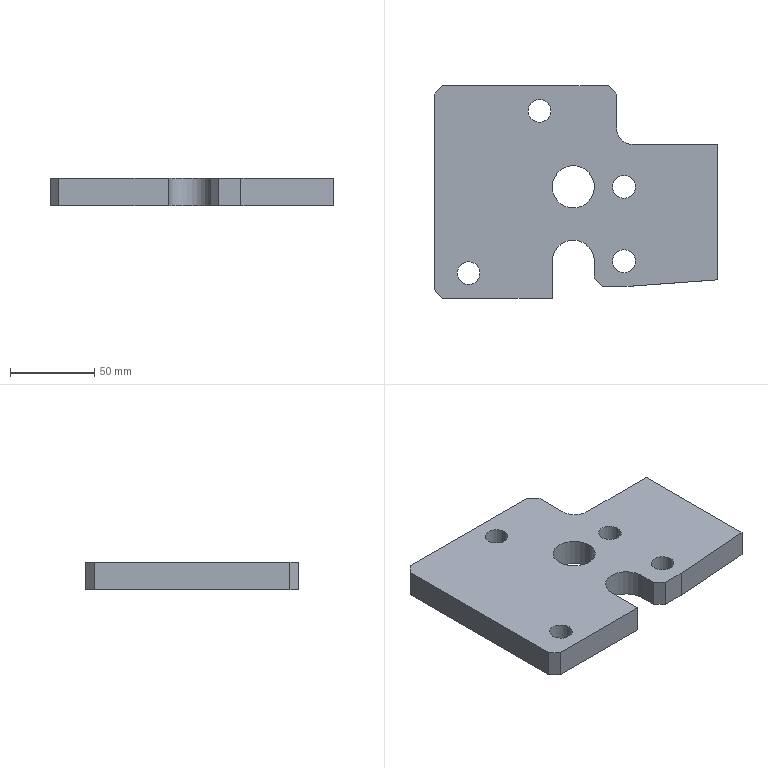Part | SolidWorks | features FlatPattern 1, SMBaseFlange 1, SheetMetal 1 | 1 solid | 28 faces | box 168 x 126 x 16 mm | volume 264942 mm3 | plane 16 | cylinder 12 | commonest cylinder face diameters 13.5 x8 25 x3 20 x1
STEP:
#1=CARTESIAN_POINT('',(-62.35,-69.,-16.));
#2=VERTEX_POINT('',#1);
#3=CARTESIAN_POINT('',(-48.85,-69.,-16.));
#4=VERTEX_POINT('',#3);
#5=CARTESIAN_POINT('',(-55.6,-69.,-16.));
#6=DIRECTION('',(0.,0.,1.));
#7=DIRECTION('',(1.,0.,0.));
#8=AXIS2_PLACEMENT_3D('',#5,#6,#7);
#9=CIRCLE('',#8,6.75);
#10=EDGE_CURVE('',#2,#4,#9,.T.);
#11=ORIENTED_EDGE('',*,*,#10,.F.);
#12=CARTESIAN_POINT('',(-62.35,-69.,0.));
#13=VERTEX_POINT('',#12);
#14=CARTESIAN_POINT('',(-62.35,-69.,-16.));
#15=DIRECTION('',(0.,0.,1.));
#16=VECTOR('',#15,1000.);
#17=LINE('',#14,#16);
#18=EDGE_CURVE('',#2,#13,#17,.T.);
#19=ORIENTED_EDGE('',*,*,#18,.T.);
#20=CARTESIAN_POINT('',(-48.85,-69.,0.));
#21=VERTEX_POINT('',#20);
#22=CARTESIAN_POINT('',(-55.6,-69.,0.));
#23=DIRECTION('',(0.,0.,1.));
#24=DIRECTION('',(1.,0.,0.));
#25=AXIS2_PLACEMENT_3D('',#22,#23,#24);
#26=CIRCLE('',#25,6.75);
#27=EDGE_CURVE('',#13,#21,#26,.T.);
#28=ORIENTED_EDGE('',*,*,#27,.T.);
#29=CARTESIAN_POINT('',(-48.85,-69.,-16.));
#30=DIRECTION('',(0.,0.,1.));
#31=VECTOR('',#30,1000.);
#32=LINE('',#29,#31);
#33=EDGE_CURVE('',#4,#21,#32,.T.);
#34=ORIENTED_EDGE('',*,*,#33,.F.);
#35=EDGE_LOOP('',(#11,#19,#28,#34));
#36=FACE_OUTER_BOUND('',#35,.T.);
#37=CARTESIAN_POINT('',(-55.6,-69.,-16.));
#38=DIRECTION('',(0.,0.,1.));
#39=DIRECTION('',(1.,0.,0.));
#40=AXIS2_PLACEMENT_3D('',#37,#38,#39);
#41=CYLINDRICAL_SURFACE('',#40,6.75);
#42=ADVANCED_FACE('',(#36),#41,.F.);
#43=CARTESIAN_POINT('',(-62.35,-25.,-16.));
#44=VERTEX_POINT('',#43);
#45=CARTESIAN_POINT('',(-48.85,-25.,-16.));
#46=VERTEX_POINT('',#45);
#47=CARTESIAN_POINT('',(-55.6,-25.,-16.));
#48=DIRECTION('',(0.,0.,1.));
#49=DIRECTION('',(1.,0.,0.));
#50=AXIS2_PLACEMENT_3D('',#47,#48,#49);
#51=CIRCLE('',#50,6.75);
#52=EDGE_CURVE('',#44,#46,#51,.T.);
#53=ORIENTED_EDGE('',*,*,#52,.F.);
#54=CARTESIAN_POINT('',(-62.35,-25.,0.));
#55=VERTEX_POINT('',#54);
#56=CARTESIAN_POINT('',(-62.35,-25.,-16.));
#57=DIRECTION('',(0.,0.,1.));
#58=VECTOR('',#57,1000.);
#59=LINE('',#56,#58);
#60=EDGE_CURVE('',#44,#55,#59,.T.);
#61=ORIENTED_EDGE('',*,*,#60,.T.);
#62=CARTESIAN_POINT('',(-48.85,-25.,0.));
#63=VERTEX_POINT('',#62);
#64=CARTESIAN_POINT('',(-55.6,-25.,0.));
#65=DIRECTION('',(0.,0.,1.));
#66=DIRECTION('',(1.,0.,0.));
#67=AXIS2_PLACEMENT_3D('',#64,#65,#66);
#68=CIRCLE('',#67,6.75);
#69=EDGE_CURVE('',#55,#63,#68,.T.);
#70=ORIENTED_EDGE('',*,*,#69,.T.);
#71=CARTESIAN_POINT('',(-48.85,-25.,-16.));
#72=DIRECTION('',(0.,0.,1.));
#73=VECTOR('',#72,1000.);
#74=LINE('',#71,#73);
#75=EDGE_CURVE('',#46,#63,#74,.T.);
#76=ORIENTED_EDGE('',*,*,#75,.F.);
#77=EDGE_LOOP('',(#53,#61,#70,#76));
#78=FACE_OUTER_BOUND('',#77,.T.);
#79=CARTESIAN_POINT('',(-55.6,-25.,-16.));
#80=DIRECTION('',(0.,0.,1.));
#81=DIRECTION('',(1.,0.,0.));
#82=AXIS2_PLACEMENT_3D('',#79,#80,#81);
#83=CYLINDRICAL_SURFACE('',#82,6.75);
#84=ADVANCED_FACE('',(#78),#83,.F.);
#85=CARTESIAN_POINT('',(-112.35,20.,-16.));
#86=VERTEX_POINT('',#85);
#87=CARTESIAN_POINT('',(-98.85,20.,-16.));
#88=VERTEX_POINT('',#87);
#89=CARTESIAN_POINT('',(-105.6,20.,-16.));
#90=DIRECTION('',(0.,0.,1.));
#91=DIRECTION('',(1.,0.,0.));
#92=AXIS2_PLACEMENT_3D('',#89,#90,#91);
#93=CIRCLE('',#92,6.75);
#94=EDGE_CURVE('',#86,#88,#93,.T.);
#95=ORIENTED_EDGE('',*,*,#94,.F.);
#96=CARTESIAN_POINT('',(-112.35,20.,0.));
#97=VERTEX_POINT('',#96);
#98=CARTESIAN_POINT('',(-112.35,20.,-16.));
#99=DIRECTION('',(0.,0.,1.));
#100=VECTOR('',#99,1000.);
#101=LINE('',#98,#100);
#102=EDGE_CURVE('',#86,#97,#101,.T.);
#103=ORIENTED_EDGE('',*,*,#102,.T.);
#104=CARTESIAN_POINT('',(-98.85,20.,0.));
#105=VERTEX_POINT('',#104);
#106=CARTESIAN_POINT('',(-105.6,20.,0.));
#107=DIRECTION('',(0.,0.,1.));
#108=DIRECTION('',(1.,0.,0.));
#109=AXIS2_PLACEMENT_3D('',#106,#107,#108);
#110=CIRCLE('',#109,6.75);
#111=EDGE_CURVE('',#97,#105,#110,.T.);
#112=ORIENTED_EDGE('',*,*,#111,.T.);
#113=CARTESIAN_POINT('',(-98.85,20.,-16.));
#114=DIRECTION('',(0.,0.,1.));
#115=VECTOR('',#114,1000.);
#116=LINE('',#113,#115);
#117=EDGE_CURVE('',#88,#105,#116,.T.);
#118=ORIENTED_EDGE('',*,*,#117,.F.);
#119=EDGE_LOOP('',(#95,#103,#112,#118));
#120=FACE_OUTER_BOUND('',#119,.T.);
#121=CARTESIAN_POINT('',(-105.6,20.,-16.));
#122=DIRECTION('',(0.,0.,1.));
#123=DIRECTION('',(1.,0.,0.));
#124=AXIS2_PLACEMENT_3D('',#121,#122,#123);
#125=CYLINDRICAL_SURFACE('',#124,6.75);
#126=ADVANCED_FACE('',(#120),#125,.F.);
#127=CARTESIAN_POINT('',(-154.35,-76.,-16.));
#128=VERTEX_POINT('',#127);
#129=CARTESIAN_POINT('',(-140.85,-76.,-16.));
#130=VERTEX_POINT('',#129);
#131=CARTESIAN_POINT('',(-147.6,-76.,-16.));
#132=DIRECTION('',(0.,0.,1.));
#133=DIRECTION('',(1.,0.,0.));
#134=AXIS2_PLACEMENT_3D('',#131,#132,#133);
#135=CIRCLE('',#134,6.75);
#136=EDGE_CURVE('',#128,#130,#135,.T.);
#137=ORIENTED_EDGE('',*,*,#136,.F.);
#138=CARTESIAN_POINT('',(-154.35,-76.,0.));
#139=VERTEX_POINT('',#138);
#140=CARTESIAN_POINT('',(-154.35,-76.,-16.));
#141=DIRECTION('',(0.,0.,1.));
#142=VECTOR('',#141,1000.);
#143=LINE('',#140,#142);
#144=EDGE_CURVE('',#128,#139,#143,.T.);
#145=ORIENTED_EDGE('',*,*,#144,.T.);
#146=CARTESIAN_POINT('',(-140.85,-76.,0.));
#147=VERTEX_POINT('',#146);
#148=CARTESIAN_POINT('',(-147.6,-76.,0.));
#149=DIRECTION('',(0.,0.,1.));
#150=DIRECTION('',(1.,0.,0.));
#151=AXIS2_PLACEMENT_3D('',#148,#149,#150);
#152=CIRCLE('',#151,6.75);
#153=EDGE_CURVE('',#139,#147,#152,.T.);
#154=ORIENTED_EDGE('',*,*,#153,.T.);
#155=CARTESIAN_POINT('',(-140.85,-76.,-16.));
#156=DIRECTION('',(0.,0.,1.));
#157=VECTOR('',#156,1000.);
#158=LINE('',#155,#157);
#159=EDGE_CURVE('',#130,#147,#158,.T.);
#160=ORIENTED_EDGE('',*,*,#159,.F.);
#161=EDGE_LOOP('',(#137,#145,#154,#160));
#162=FACE_OUTER_BOUND('',#161,.T.);
#163=CARTESIAN_POINT('',(-147.6,-76.,-16.));
#164=DIRECTION('',(0.,0.,1.));
#165=DIRECTION('',(1.,0.,0.));
#166=AXIS2_PLACEMENT_3D('',#163,#164,#165);
#167=CYLINDRICAL_SURFACE('',#166,6.75);
#168=ADVANCED_FACE('',(#162),#167,.F.);
#169=CARTESIAN_POINT('',(-98.1,-25.,-16.));
#170=VERTEX_POINT('',#169);
#171=CARTESIAN_POINT('',(-73.1,-25.,-16.));
#172=VERTEX_POINT('',#171);
#173=CARTESIAN_POINT('',(-85.6,-25.,-16.));
#174=DIRECTION('',(0.,0.,1.));
#175=DIRECTION('',(1.,0.,0.));
#176=AXIS2_PLACEMENT_3D('',#173,#174,#175);
#177=CIRCLE('',#176,12.5);
#178=EDGE_CURVE('',#170,#172,#177,.T.);
#179=ORIENTED_EDGE('',*,*,#178,.F.);
#180=CARTESIAN_POINT('',(-98.1,-25.,0.));
#181=VERTEX_POINT('',#180);
#182=CARTESIAN_POINT('',(-98.1,-25.,-16.));
#183=DIRECTION('',(0.,0.,1.));
#184=VECTOR('',#183,1000.);
#185=LINE('',#182,#184);
#186=EDGE_CURVE('',#170,#181,#185,.T.);
#187=ORIENTED_EDGE('',*,*,#186,.T.);
#188=CARTESIAN_POINT('',(-73.1,-25.,0.));
#189=VERTEX_POINT('',#188);
#190=CARTESIAN_POINT('',(-85.6,-25.,0.));
#191=DIRECTION('',(0.,0.,1.));
#192=DIRECTION('',(1.,0.,0.));
#193=AXIS2_PLACEMENT_3D('',#190,#191,#192);
#194=CIRCLE('',#193,12.5);
#195=EDGE_CURVE('',#181,#189,#194,.T.);
#196=ORIENTED_EDGE('',*,*,#195,.T.);
#197=CARTESIAN_POINT('',(-73.1,-25.,-16.));
#198=DIRECTION('',(0.,0.,1.));
#199=VECTOR('',#198,1000.);
#200=LINE('',#197,#199);
#201=EDGE_CURVE('',#172,#189,#200,.T.);
#202=ORIENTED_EDGE('',*,*,#201,.F.);
#203=EDGE_LOOP('',(#179,#187,#196,#202));
#204=FACE_OUTER_BOUND('',#203,.T.);
#205=CARTESIAN_POINT('',(-85.6,-25.,-16.));
#206=DIRECTION('',(0.,0.,1.));
#207=DIRECTION('',(1.,0.,0.));
#208=AXIS2_PLACEMENT_3D('',#205,#206,#207);
#209=CYLINDRICAL_SURFACE('',#208,12.5);
#210=ADVANCED_FACE('',(#204),#209,.F.);
#211=CARTESIAN_POINT('',(0.,0.,0.));
#212=VERTEX_POINT('',#211);
#213=CARTESIAN_POINT('',(-50.,0.,0.));
#214=VERTEX_POINT('',#213);
#215=CARTESIAN_POINT('',(-50.,0.,0.));
#216=DIRECTION('',(-1.,0.,0.));
#217=VECTOR('',#216,1000.);
#218=LINE('',#215,#217);
#219=EDGE_CURVE('',#212,#214,#218,.T.);
#220=ORIENTED_EDGE('',*,*,#219,.F.);
#221=CARTESIAN_POINT('',(0.,0.,-16.));
#222=VERTEX_POINT('',#221);
#223=CARTESIAN_POINT('',(0.,0.,-16.));
#224=DIRECTION('',(0.,0.,1.));
#225=VECTOR('',#224,1000.);
#226=LINE('',#223,#225);
#227=EDGE_CURVE('',#222,#212,#226,.T.);
#228=ORIENTED_EDGE('',*,*,#227,.F.);
#229=CARTESIAN_POINT('',(-50.,0.,-16.));
#230=VERTEX_POINT('',#229);
#231=CARTESIAN_POINT('',(-50.,0.,-16.));
#232=DIRECTION('',(-1.,0.,0.));
#233=VECTOR('',#232,1000.);
#234=LINE('',#231,#233);
#235=EDGE_CURVE('',#222,#230,#234,.T.);
#236=ORIENTED_EDGE('',*,*,#235,.T.);
#237=CARTESIAN_POINT('',(-50.,0.,-16.));
#238=DIRECTION('',(0.,0.,1.));
#239=VECTOR('',#238,1000.);
#240=LINE('',#237,#239);
#241=EDGE_CURVE('',#230,#214,#240,.T.);
#242=ORIENTED_EDGE('',*,*,#241,.T.);
#243=EDGE_LOOP('',(#220,#228,#236,#242));
#244=FACE_OUTER_BOUND('',#243,.T.);
#245=CARTESIAN_POINT('',(-50.,0.,-16.));
#246=DIRECTION('',(0.,1.,0.));
#247=DIRECTION('',(-1.,0.,0.));
#248=AXIS2_PLACEMENT_3D('',#245,#246,#247);
#249=PLANE('',#248);
#250=ADVANCED_FACE('',(#244),#249,.T.);
#251=CARTESIAN_POINT('',(0.,-80.,0.));
#252=VERTEX_POINT('',#251);
#253=CARTESIAN_POINT('',(0.,0.,0.));
#254=DIRECTION('',(0.,1.,0.));
#255=VECTOR('',#254,1000.);
#256=LINE('',#253,#255);
#257=EDGE_CURVE('',#252,#212,#256,.T.);
#258=ORIENTED_EDGE('',*,*,#257,.F.);
#259=CARTESIAN_POINT('',(0.,-80.,-16.));
#260=VERTEX_POINT('',#259);
#261=CARTESIAN_POINT('',(0.,-80.,-16.));
#262=DIRECTION('',(0.,0.,1.));
#263=VECTOR('',#262,1000.);
#264=LINE('',#261,#263);
#265=EDGE_CURVE('',#260,#252,#264,.T.);
#266=ORIENTED_EDGE('',*,*,#265,.F.);
#267=CARTESIAN_POINT('',(0.,0.,-16.));
#268=DIRECTION('',(0.,1.,0.));
#269=VECTOR('',#268,1000.);
#270=LINE('',#267,#269);
#271=EDGE_CURVE('',#260,#222,#270,.T.);
#272=ORIENTED_EDGE('',*,*,#271,.T.);
#273=ORIENTED_EDGE('',*,*,#227,.T.);
#274=EDGE_LOOP('',(#258,#266,#272,#273));
#275=FACE_OUTER_BOUND('',#274,.T.);
#276=CARTESIAN_POINT('',(0.,0.,-16.));
#277=DIRECTION('',(1.,0.,0.));
#278=DIRECTION('',(0.,0.,-1.));
#279=AXIS2_PLACEMENT_3D('',#276,#277,#278);
#280=PLANE('',#279);
#281=ADVANCED_FACE('',(#275),#280,.T.);
#282=CARTESIAN_POINT('',(-55.,-84.,0.));
#283=VERTEX_POINT('',#282);
#284=CARTESIAN_POINT('',(-55.,-84.,0.));
#285=DIRECTION('',(0.9974,0.07254,0.));
#286=VECTOR('',#285,1000.);
#287=LINE('',#284,#286);
#288=EDGE_CURVE('',#283,#252,#287,.T.);
#289=ORIENTED_EDGE('',*,*,#288,.F.);
#290=CARTESIAN_POINT('',(-55.,-84.,-16.));
#291=VERTEX_POINT('',#290);
#292=CARTESIAN_POINT('',(-55.,-84.,-16.));
#293=DIRECTION('',(0.,0.,1.));
#294=VECTOR('',#293,1000.);
#295=LINE('',#292,#294);
#296=EDGE_CURVE('',#291,#283,#295,.T.);
#297=ORIENTED_EDGE('',*,*,#296,.F.);
#298=CARTESIAN_POINT('',(-55.,-84.,-16.));
#299=DIRECTION('',(0.9974,0.07254,0.));
#300=VECTOR('',#299,1000.);
#301=LINE('',#298,#300);
#302=EDGE_CURVE('',#291,#260,#301,.T.);
#303=ORIENTED_EDGE('',*,*,#302,.T.);
#304=ORIENTED_EDGE('',*,*,#265,.T.);
#305=EDGE_LOOP('',(#289,#297,#303,#304));
#306=FACE_OUTER_BOUND('',#305,.T.);
#307=CARTESIAN_POINT('',(-55.,-84.,-16.));
#308=DIRECTION('',(0.07254,-0.9974,0.));
#309=DIRECTION('',(0.9974,0.07254,0.));
#310=AXIS2_PLACEMENT_3D('',#307,#308,#309);
#311=PLANE('',#310);
#312=ADVANCED_FACE('',(#306),#311,.T.);
#313=CARTESIAN_POINT('',(-68.1,-84.,0.));
#314=VERTEX_POINT('',#313);
#315=CARTESIAN_POINT('',(-68.1,-84.,0.));
#316=DIRECTION('',(1.,0.,0.));
#317=VECTOR('',#316,1000.);
#318=LINE('',#315,#317);
#319=EDGE_CURVE('',#314,#283,#318,.T.);
#320=ORIENTED_EDGE('',*,*,#319,.F.);
#321=CARTESIAN_POINT('',(-68.1,-84.,-16.));
#322=VERTEX_POINT('',#321);
#323=CARTESIAN_POINT('',(-68.1,-84.,-16.));
#324=DIRECTION('',(0.,0.,1.));
#325=VECTOR('',#324,1000.);
#326=LINE('',#323,#325);
#327=EDGE_CURVE('',#322,#314,#326,.T.);
#328=ORIENTED_EDGE('',*,*,#327,.F.);
#329=CARTESIAN_POINT('',(-68.1,-84.,-16.));
#330=DIRECTION('',(1.,0.,0.));
#331=VECTOR('',#330,1000.);
#332=LINE('',#329,#331);
#333=EDGE_CURVE('',#322,#291,#332,.T.);
#334=ORIENTED_EDGE('',*,*,#333,.T.);
#335=ORIENTED_EDGE('',*,*,#296,.T.);
#336=EDGE_LOOP('',(#320,#328,#334,#335));
#337=FACE_OUTER_BOUND('',#336,.T.);
#338=CARTESIAN_POINT('',(-68.1,-84.,-16.));
#339=DIRECTION('',(0.,-1.,0.));
#340=DIRECTION('',(0.,0.,-1.));
#341=AXIS2_PLACEMENT_3D('',#338,#339,#340);
#342=PLANE('',#341);
#343=ADVANCED_FACE('',(#337),#342,.T.);
#344=CARTESIAN_POINT('',(-73.1,-79.,0.));
#345=VERTEX_POINT('',#344);
#346=CARTESIAN_POINT('',(-73.1,-79.,0.));
#347=DIRECTION('',(0.7071,-0.7071,0.));
#348=VECTOR('',#347,1000.);
#349=LINE('',#346,#348);
#350=EDGE_CURVE('',#345,#314,#349,.T.);
#351=ORIENTED_EDGE('',*,*,#350,.F.);
#352=CARTESIAN_POINT('',(-73.1,-79.,-16.));
#353=VERTEX_POINT('',#352);
#354=CARTESIAN_POINT('',(-73.1,-79.,-16.));
#355=DIRECTION('',(0.,0.,1.));
#356=VECTOR('',#355,1000.);
#357=LINE('',#354,#356);
#358=EDGE_CURVE('',#353,#345,#357,.T.);
#359=ORIENTED_EDGE('',*,*,#358,.F.);
#360=CARTESIAN_POINT('',(-73.1,-79.,-16.));
#361=DIRECTION('',(0.7071,-0.7071,0.));
#362=VECTOR('',#361,1000.);
#363=LINE('',#360,#362);
#364=EDGE_CURVE('',#353,#322,#363,.T.);
#365=ORIENTED_EDGE('',*,*,#364,.T.);
#366=ORIENTED_EDGE('',*,*,#327,.T.);
#367=EDGE_LOOP('',(#351,#359,#365,#366));
#368=FACE_OUTER_BOUND('',#367,.T.);
#369=CARTESIAN_POINT('',(-73.1,-79.,-16.));
#370=DIRECTION('',(-0.7071,-0.7071,0.));
#371=DIRECTION('',(0.7071,-0.7071,0.));
#372=AXIS2_PLACEMENT_3D('',#369,#370,#371);
#373=PLANE('',#372);
#374=ADVANCED_FACE('',(#368),#373,.T.);
#375=CARTESIAN_POINT('',(-73.1,-69.,0.));
#376=VERTEX_POINT('',#375);
#377=CARTESIAN_POINT('',(-73.1,-69.,0.));
#378=DIRECTION('',(0.,-1.,0.));
#379=VECTOR('',#378,1000.);
#380=LINE('',#377,#379);
#381=EDGE_CURVE('',#376,#345,#380,.T.);
#382=ORIENTED_EDGE('',*,*,#381,.F.);
#383=CARTESIAN_POINT('',(-73.1,-69.,-16.));
#384=VERTEX_POINT('',#383);
#385=CARTESIAN_POINT('',(-73.1,-69.,-16.));
#386=DIRECTION('',(0.,0.,1.));
#387=VECTOR('',#386,1000.);
#388=LINE('',#385,#387);
#389=EDGE_CURVE('',#384,#376,#388,.T.);
#390=ORIENTED_EDGE('',*,*,#389,.F.);
#391=CARTESIAN_POINT('',(-73.1,-69.,-16.));
#392=DIRECTION('',(0.,-1.,0.));
#393=VECTOR('',#392,1000.);
#394=LINE('',#391,#393);
#395=EDGE_CURVE('',#384,#353,#394,.T.);
#396=ORIENTED_EDGE('',*,*,#395,.T.);
#397=ORIENTED_EDGE('',*,*,#358,.T.);
#398=EDGE_LOOP('',(#382,#390,#396,#397));
#399=FACE_OUTER_BOUND('',#398,.T.);
#400=CARTESIAN_POINT('',(-73.1,-69.,-16.));
#401=DIRECTION('',(-1.,0.,0.));
#402=DIRECTION('',(0.,0.,1.));
#403=AXIS2_PLACEMENT_3D('',#400,#401,#402);
#404=PLANE('',#403);
#405=ADVANCED_FACE('',(#399),#404,.T.);
#406=CARTESIAN_POINT('',(-98.1,-69.,0.));
#407=VERTEX_POINT('',#406);
#408=CARTESIAN_POINT('',(-85.6,-69.,0.));
#409=DIRECTION('',(0.,0.,-1.));
#410=DIRECTION('',(1.,0.,0.));
#411=AXIS2_PLACEMENT_3D('',#408,#409,#410);
#412=CIRCLE('',#411,12.5);
#413=EDGE_CURVE('',#407,#376,#412,.T.);
#414=ORIENTED_EDGE('',*,*,#413,.F.);
#415=CARTESIAN_POINT('',(-98.1,-69.,-16.));
#416=VERTEX_POINT('',#415);
#417=CARTESIAN_POINT('',(-98.1,-69.,-16.));
#418=DIRECTION('',(0.,0.,1.));
#419=VECTOR('',#418,1000.);
#420=LINE('',#417,#419);
#421=EDGE_CURVE('',#416,#407,#420,.T.);
#422=ORIENTED_EDGE('',*,*,#421,.F.);
#423=CARTESIAN_POINT('',(-85.6,-69.,-16.));
#424=DIRECTION('',(0.,0.,-1.));
#425=DIRECTION('',(1.,0.,0.));
#426=AXIS2_PLACEMENT_3D('',#423,#424,#425);
#427=CIRCLE('',#426,12.5);
#428=EDGE_CURVE('',#416,#384,#427,.T.);
#429=ORIENTED_EDGE('',*,*,#428,.T.);
#430=ORIENTED_EDGE('',*,*,#389,.T.);
#431=EDGE_LOOP('',(#414,#422,#429,#430));
#432=FACE_OUTER_BOUND('',#431,.T.);
#433=CARTESIAN_POINT('',(-85.6,-69.,-16.));
#434=DIRECTION('',(0.,0.,1.));
#435=DIRECTION('',(1.,0.,0.));
#436=AXIS2_PLACEMENT_3D('',#433,#434,#435);
#437=CYLINDRICAL_SURFACE('',#436,12.5);
#438=ADVANCED_FACE('',(#432),#437,.F.);
#439=CARTESIAN_POINT('',(-98.1,-91.,0.));
#440=VERTEX_POINT('',#439);
#441=CARTESIAN_POINT('',(-98.1,-91.,0.));
#442=DIRECTION('',(0.,1.,0.));
#443=VECTOR('',#442,1000.);
#444=LINE('',#441,#443);
#445=EDGE_CURVE('',#440,#407,#444,.T.);
#446=ORIENTED_EDGE('',*,*,#445,.F.);
#447=CARTESIAN_POINT('',(-98.1,-91.,-16.));
#448=VERTEX_POINT('',#447);
#449=CARTESIAN_POINT('',(-98.1,-91.,-16.));
#450=DIRECTION('',(0.,0.,1.));
#451=VECTOR('',#450,1000.);
#452=LINE('',#449,#451);
#453=EDGE_CURVE('',#448,#440,#452,.T.);
#454=ORIENTED_EDGE('',*,*,#453,.F.);
#455=CARTESIAN_POINT('',(-98.1,-91.,-16.));
#456=DIRECTION('',(0.,1.,0.));
#457=VECTOR('',#456,1000.);
#458=LINE('',#455,#457);
#459=EDGE_CURVE('',#448,#416,#458,.T.);
#460=ORIENTED_EDGE('',*,*,#459,.T.);
#461=ORIENTED_EDGE('',*,*,#421,.T.);
#462=EDGE_LOOP('',(#446,#454,#460,#461));
#463=FACE_OUTER_BOUND('',#462,.T.);
#464=CARTESIAN_POINT('',(-98.1,-91.,-16.));
#465=DIRECTION('',(1.,0.,0.));
#466=DIRECTION('',(0.,1.,0.));
#467=AXIS2_PLACEMENT_3D('',#464,#465,#466);
#468=PLANE('',#467);
#469=ADVANCED_FACE('',(#463),#468,.T.);
#470=CARTESIAN_POINT('',(-163.,-91.,0.));
#471=VERTEX_POINT('',#470);
#472=CARTESIAN_POINT('',(-163.,-91.,0.));
#473=DIRECTION('',(1.,0.,0.));
#474=VECTOR('',#473,1000.);
#475=LINE('',#472,#474);
#476=EDGE_CURVE('',#471,#440,#475,.T.);
#477=ORIENTED_EDGE('',*,*,#476,.F.);
#478=CARTESIAN_POINT('',(-163.,-91.,-16.));
#479=VERTEX_POINT('',#478);
#480=CARTESIAN_POINT('',(-163.,-91.,-16.));
#481=DIRECTION('',(0.,0.,1.));
#482=VECTOR('',#481,1000.);
#483=LINE('',#480,#482);
#484=EDGE_CURVE('',#479,#471,#483,.T.);
#485=ORIENTED_EDGE('',*,*,#484,.F.);
#486=CARTESIAN_POINT('',(-163.,-91.,-16.));
#487=DIRECTION('',(1.,0.,0.));
#488=VECTOR('',#487,1000.);
#489=LINE('',#486,#488);
#490=EDGE_CURVE('',#479,#448,#489,.T.);
#491=ORIENTED_EDGE('',*,*,#490,.T.);
#492=ORIENTED_EDGE('',*,*,#453,.T.);
#493=EDGE_LOOP('',(#477,#485,#491,#492));
#494=FACE_OUTER_BOUND('',#493,.T.);
#495=CARTESIAN_POINT('',(-163.,-91.,-16.));
#496=DIRECTION('',(0.,-1.,0.));
#497=DIRECTION('',(0.,0.,-1.));
#498=AXIS2_PLACEMENT_3D('',#495,#496,#497);
#499=PLANE('',#498);
#500=ADVANCED_FACE('',(#494),#499,.T.);
#501=CARTESIAN_POINT('',(-168.,-86.,0.));
#502=VERTEX_POINT('',#501);
#503=CARTESIAN_POINT('',(-168.,-86.,0.));
#504=DIRECTION('',(0.7071,-0.7071,0.));
#505=VECTOR('',#504,1000.);
#506=LINE('',#503,#505);
#507=EDGE_CURVE('',#502,#471,#506,.T.);
#508=ORIENTED_EDGE('',*,*,#507,.F.);
#509=CARTESIAN_POINT('',(-168.,-86.,-16.));
#510=VERTEX_POINT('',#509);
#511=CARTESIAN_POINT('',(-168.,-86.,-16.));
#512=DIRECTION('',(0.,0.,1.));
#513=VECTOR('',#512,1000.);
#514=LINE('',#511,#513);
#515=EDGE_CURVE('',#510,#502,#514,.T.);
#516=ORIENTED_EDGE('',*,*,#515,.F.);
#517=CARTESIAN_POINT('',(-168.,-86.,-16.));
#518=DIRECTION('',(0.7071,-0.7071,0.));
#519=VECTOR('',#518,1000.);
#520=LINE('',#517,#519);
#521=EDGE_CURVE('',#510,#479,#520,.T.);
#522=ORIENTED_EDGE('',*,*,#521,.T.);
#523=ORIENTED_EDGE('',*,*,#484,.T.);
#524=EDGE_LOOP('',(#508,#516,#522,#523));
#525=FACE_OUTER_BOUND('',#524,.T.);
#526=CARTESIAN_POINT('',(-168.,-86.,-16.));
#527=DIRECTION('',(-0.7071,-0.7071,0.));
#528=DIRECTION('',(0.7071,-0.7071,0.));
#529=AXIS2_PLACEMENT_3D('',#526,#527,#528);
#530=PLANE('',#529);
#531=ADVANCED_FACE('',(#525),#530,.T.);
#532=CARTESIAN_POINT('',(-168.,30.,0.));
#533=VERTEX_POINT('',#532);
#534=CARTESIAN_POINT('',(-168.,-86.,0.));
#535=DIRECTION('',(0.,-1.,0.));
#536=VECTOR('',#535,1000.);
#537=LINE('',#534,#536);
#538=EDGE_CURVE('',#533,#502,#537,.T.);
#539=ORIENTED_EDGE('',*,*,#538,.F.);
#540=CARTESIAN_POINT('',(-168.,30.,-16.));
#541=VERTEX_POINT('',#540);
#542=CARTESIAN_POINT('',(-168.,30.,-16.));
#543=DIRECTION('',(0.,0.,1.));
#544=VECTOR('',#543,1000.);
#545=LINE('',#542,#544);
#546=EDGE_CURVE('',#541,#533,#545,.T.);
#547=ORIENTED_EDGE('',*,*,#546,.F.);
#548=CARTESIAN_POINT('',(-168.,-86.,-16.));
#549=DIRECTION('',(0.,-1.,0.));
#550=VECTOR('',#549,1000.);
#551=LINE('',#548,#550);
#552=EDGE_CURVE('',#541,#510,#551,.T.);
#553=ORIENTED_EDGE('',*,*,#552,.T.);
#554=ORIENTED_EDGE('',*,*,#515,.T.);
#555=EDGE_LOOP('',(#539,#547,#553,#554));
#556=FACE_OUTER_BOUND('',#555,.T.);
#557=CARTESIAN_POINT('',(-168.,-86.,-16.));
#558=DIRECTION('',(-1.,0.,0.));
#559=DIRECTION('',(0.,-1.,0.));
#560=AXIS2_PLACEMENT_3D('',#557,#558,#559);
#561=PLANE('',#560);
#562=ADVANCED_FACE('',(#556),#561,.T.);
#563=CARTESIAN_POINT('',(-163.,35.,0.));
#564=VERTEX_POINT('',#563);
#565=CARTESIAN_POINT('',(-168.,30.,0.));
#566=DIRECTION('',(-0.7071,-0.7071,0.));
#567=VECTOR('',#566,1000.);
#568=LINE('',#565,#567);
#569=EDGE_CURVE('',#564,#533,#568,.T.);
#570=ORIENTED_EDGE('',*,*,#569,.F.);
#571=CARTESIAN_POINT('',(-163.,35.,-16.));
#572=VERTEX_POINT('',#571);
#573=CARTESIAN_POINT('',(-163.,35.,-16.));
#574=DIRECTION('',(0.,0.,1.));
#575=VECTOR('',#574,1000.);
#576=LINE('',#573,#575);
#577=EDGE_CURVE('',#572,#564,#576,.T.);
#578=ORIENTED_EDGE('',*,*,#577,.F.);
#579=CARTESIAN_POINT('',(-168.,30.,-16.));
#580=DIRECTION('',(-0.7071,-0.7071,0.));
#581=VECTOR('',#580,1000.);
#582=LINE('',#579,#581);
#583=EDGE_CURVE('',#572,#541,#582,.T.);
#584=ORIENTED_EDGE('',*,*,#583,.T.);
#585=ORIENTED_EDGE('',*,*,#546,.T.);
#586=EDGE_LOOP('',(#570,#578,#584,#585));
#587=FACE_OUTER_BOUND('',#586,.T.);
#588=CARTESIAN_POINT('',(-168.,30.,-16.));
#589=DIRECTION('',(-0.7071,0.7071,0.));
#590=DIRECTION('',(-0.7071,-0.7071,0.));
#591=AXIS2_PLACEMENT_3D('',#588,#589,#590);
#592=PLANE('',#591);
#593=ADVANCED_FACE('',(#587),#592,.T.);
#594=CARTESIAN_POINT('',(-65.,35.,0.));
#595=VERTEX_POINT('',#594);
#596=CARTESIAN_POINT('',(-163.,35.,0.));
#597=DIRECTION('',(-1.,0.,0.));
#598=VECTOR('',#597,1000.);
#599=LINE('',#596,#598);
#600=EDGE_CURVE('',#595,#564,#599,.T.);
#601=ORIENTED_EDGE('',*,*,#600,.F.);
#602=CARTESIAN_POINT('',(-65.,35.,-16.));
#603=VERTEX_POINT('',#602);
#604=CARTESIAN_POINT('',(-65.,35.,-16.));
#605=DIRECTION('',(0.,0.,1.));
#606=VECTOR('',#605,1000.);
#607=LINE('',#604,#606);
#608=EDGE_CURVE('',#603,#595,#607,.T.);
#609=ORIENTED_EDGE('',*,*,#608,.F.);
#610=CARTESIAN_POINT('',(-163.,35.,-16.));
#611=DIRECTION('',(-1.,0.,0.));
#612=VECTOR('',#611,1000.);
#613=LINE('',#610,#612);
#614=EDGE_CURVE('',#603,#572,#613,.T.);
#615=ORIENTED_EDGE('',*,*,#614,.T.);
#616=ORIENTED_EDGE('',*,*,#577,.T.);
#617=EDGE_LOOP('',(#601,#609,#615,#616));
#618=FACE_OUTER_BOUND('',#617,.T.);
#619=CARTESIAN_POINT('',(-163.,35.,-16.));
#620=DIRECTION('',(0.,1.,0.));
#621=DIRECTION('',(0.,0.,1.));
#622=AXIS2_PLACEMENT_3D('',#619,#620,#621);
#623=PLANE('',#622);
#624=ADVANCED_FACE('',(#618),#623,.T.);
#625=CARTESIAN_POINT('',(-60.,30.,0.));
#626=VERTEX_POINT('',#625);
#627=CARTESIAN_POINT('',(-65.,35.,0.));
#628=DIRECTION('',(-0.7071,0.7071,0.));
#629=VECTOR('',#628,1000.);
#630=LINE('',#627,#629);
#631=EDGE_CURVE('',#626,#595,#630,.T.);
#632=ORIENTED_EDGE('',*,*,#631,.F.);
#633=CARTESIAN_POINT('',(-60.,30.,-16.));
#634=VERTEX_POINT('',#633);
#635=CARTESIAN_POINT('',(-60.,30.,-16.));
#636=DIRECTION('',(0.,0.,1.));
#637=VECTOR('',#636,1000.);
#638=LINE('',#635,#637);
#639=EDGE_CURVE('',#634,#626,#638,.T.);
#640=ORIENTED_EDGE('',*,*,#639,.F.);
#641=CARTESIAN_POINT('',(-65.,35.,-16.));
#642=DIRECTION('',(-0.7071,0.7071,0.));
#643=VECTOR('',#642,1000.);
#644=LINE('',#641,#643);
#645=EDGE_CURVE('',#634,#603,#644,.T.);
#646=ORIENTED_EDGE('',*,*,#645,.T.);
#647=ORIENTED_EDGE('',*,*,#608,.T.);
#648=EDGE_LOOP('',(#632,#640,#646,#647));
#649=FACE_OUTER_BOUND('',#648,.T.);
#650=CARTESIAN_POINT('',(-65.,35.,-16.));
#651=DIRECTION('',(0.7071,0.7071,0.));
#652=DIRECTION('',(-0.7071,0.7071,0.));
#653=AXIS2_PLACEMENT_3D('',#650,#651,#652);
#654=PLANE('',#653);
#655=ADVANCED_FACE('',(#649),#654,.T.);
#656=CARTESIAN_POINT('',(-60.,10.,0.));
#657=VERTEX_POINT('',#656);
#658=CARTESIAN_POINT('',(-60.,30.,0.));
#659=DIRECTION('',(0.,1.,0.));
#660=VECTOR('',#659,1000.);
#661=LINE('',#658,#660);
#662=EDGE_CURVE('',#657,#626,#661,.T.);
#663=ORIENTED_EDGE('',*,*,#662,.F.);
#664=CARTESIAN_POINT('',(-60.,10.,-16.));
#665=VERTEX_POINT('',#664);
#666=CARTESIAN_POINT('',(-60.,10.,-16.));
#667=DIRECTION('',(0.,0.,1.));
#668=VECTOR('',#667,1000.);
#669=LINE('',#666,#668);
#670=EDGE_CURVE('',#665,#657,#669,.T.);
#671=ORIENTED_EDGE('',*,*,#670,.F.);
#672=CARTESIAN_POINT('',(-60.,30.,-16.));
#673=DIRECTION('',(0.,1.,0.));
#674=VECTOR('',#673,1000.);
#675=LINE('',#672,#674);
#676=EDGE_CURVE('',#665,#634,#675,.T.);
#677=ORIENTED_EDGE('',*,*,#676,.T.);
#678=ORIENTED_EDGE('',*,*,#639,.T.);
#679=EDGE_LOOP('',(#663,#671,#677,#678));
#680=FACE_OUTER_BOUND('',#679,.T.);
#681=CARTESIAN_POINT('',(-60.,30.,-16.));
#682=DIRECTION('',(1.,0.,0.));
#683=DIRECTION('',(0.,1.,0.));
#684=AXIS2_PLACEMENT_3D('',#681,#682,#683);
#685=PLANE('',#684);
#686=ADVANCED_FACE('',(#680),#685,.T.);
#687=CARTESIAN_POINT('',(-50.,10.,0.));
#688=DIRECTION('',(0.,0.,-1.));
#689=DIRECTION('',(1.,0.,0.));
#690=AXIS2_PLACEMENT_3D('',#687,#688,#689);
#691=CIRCLE('',#690,10.);
#692=EDGE_CURVE('',#214,#657,#691,.T.);
#693=ORIENTED_EDGE('',*,*,#692,.F.);
#694=ORIENTED_EDGE('',*,*,#241,.F.);
#695=CARTESIAN_POINT('',(-50.,10.,-16.));
#696=DIRECTION('',(0.,0.,-1.));
#697=DIRECTION('',(1.,0.,0.));
#698=AXIS2_PLACEMENT_3D('',#695,#696,#697);
#699=CIRCLE('',#698,10.);
#700=EDGE_CURVE('',#230,#665,#699,.T.);
#701=ORIENTED_EDGE('',*,*,#700,.T.);
#702=ORIENTED_EDGE('',*,*,#670,.T.);
#703=EDGE_LOOP('',(#693,#694,#701,#702));
#704=FACE_OUTER_BOUND('',#703,.T.);
#705=CARTESIAN_POINT('',(-50.,10.,-16.));
#706=DIRECTION('',(0.,0.,1.));
#707=DIRECTION('',(1.,0.,0.));
#708=AXIS2_PLACEMENT_3D('',#705,#706,#707);
#709=CYLINDRICAL_SURFACE('',#708,10.);
#710=ADVANCED_FACE('',(#704),#709,.F.);
#711=CARTESIAN_POINT('',(-55.6,-69.,-16.));
#712=DIRECTION('',(0.,0.,1.));
#713=DIRECTION('',(1.,0.,0.));
#714=AXIS2_PLACEMENT_3D('',#711,#712,#713);
#715=CIRCLE('',#714,6.75);
#716=EDGE_CURVE('',#4,#2,#715,.T.);
#717=ORIENTED_EDGE('',*,*,#716,.T.);
#718=ORIENTED_EDGE('',*,*,#10,.T.);
#719=EDGE_LOOP('',(#717,#718));
#720=FACE_BOUND('',#719,.T.);
#721=CARTESIAN_POINT('',(-55.6,-25.,-16.));
#722=DIRECTION('',(0.,0.,1.));
#723=DIRECTION('',(1.,0.,0.));
#724=AXIS2_PLACEMENT_3D('',#721,#722,#723);
#725=CIRCLE('',#724,6.75);
#726=EDGE_CURVE('',#46,#44,#725,.T.);
#727=ORIENTED_EDGE('',*,*,#726,.T.);
#728=ORIENTED_EDGE('',*,*,#52,.T.);
#729=EDGE_LOOP('',(#727,#728));
#730=FACE_BOUND('',#729,.T.);
#731=CARTESIAN_POINT('',(-105.6,20.,-16.));
#732=DIRECTION('',(0.,0.,1.));
#733=DIRECTION('',(1.,0.,0.));
#734=AXIS2_PLACEMENT_3D('',#731,#732,#733);
#735=CIRCLE('',#734,6.75);
#736=EDGE_CURVE('',#88,#86,#735,.T.);
#737=ORIENTED_EDGE('',*,*,#736,.T.);
#738=ORIENTED_EDGE('',*,*,#94,.T.);
#739=EDGE_LOOP('',(#737,#738));
#740=FACE_BOUND('',#739,.T.);
#741=CARTESIAN_POINT('',(-147.6,-76.,-16.));
#742=DIRECTION('',(0.,0.,1.));
#743=DIRECTION('',(1.,0.,0.));
#744=AXIS2_PLACEMENT_3D('',#741,#742,#743);
#745=CIRCLE('',#744,6.75);
#746=EDGE_CURVE('',#130,#128,#745,.T.);
#747=ORIENTED_EDGE('',*,*,#746,.T.);
#748=ORIENTED_EDGE('',*,*,#136,.T.);
#749=EDGE_LOOP('',(#747,#748));
#750=FACE_BOUND('',#749,.T.);
#751=CARTESIAN_POINT('',(-85.6,-25.,-16.));
#752=DIRECTION('',(0.,0.,1.));
#753=DIRECTION('',(1.,0.,0.));
#754=AXIS2_PLACEMENT_3D('',#751,#752,#753);
#755=CIRCLE('',#754,12.5);
#756=EDGE_CURVE('',#172,#170,#755,.T.);
#757=ORIENTED_EDGE('',*,*,#756,.T.);
#758=ORIENTED_EDGE('',*,*,#178,.T.);
#759=EDGE_LOOP('',(#757,#758));
#760=FACE_BOUND('',#759,.T.);
#761=ORIENTED_EDGE('',*,*,#235,.F.);
#762=ORIENTED_EDGE('',*,*,#271,.F.);
#763=ORIENTED_EDGE('',*,*,#302,.F.);
#764=ORIENTED_EDGE('',*,*,#333,.F.);
#765=ORIENTED_EDGE('',*,*,#364,.F.);
#766=ORIENTED_EDGE('',*,*,#395,.F.);
#767=ORIENTED_EDGE('',*,*,#428,.F.);
#768=ORIENTED_EDGE('',*,*,#459,.F.);
#769=ORIENTED_EDGE('',*,*,#490,.F.);
#770=ORIENTED_EDGE('',*,*,#521,.F.);
#771=ORIENTED_EDGE('',*,*,#552,.F.);
#772=ORIENTED_EDGE('',*,*,#583,.F.);
#773=ORIENTED_EDGE('',*,*,#614,.F.);
#774=ORIENTED_EDGE('',*,*,#645,.F.);
#775=ORIENTED_EDGE('',*,*,#676,.F.);
#776=ORIENTED_EDGE('',*,*,#700,.F.);
#777=EDGE_LOOP('',(#761,#762,#763,#764,#765,#766,#767,#768,#769,#770,#771,#772,#773,#774,#775,#776));
#778=FACE_OUTER_BOUND('',#777,.T.);
#779=CARTESIAN_POINT('',(-85.6,-69.,-16.));
#780=DIRECTION('',(0.,0.,1.));
#781=DIRECTION('',(1.,0.,0.));
#782=AXIS2_PLACEMENT_3D('',#779,#780,#781);
#783=PLANE('',#782);
#784=ADVANCED_FACE('',(#720,#730,#740,#750,#760,#778),#783,.F.);
#785=CARTESIAN_POINT('',(-55.6,-69.,0.));
#786=DIRECTION('',(0.,0.,1.));
#787=DIRECTION('',(1.,0.,0.));
#788=AXIS2_PLACEMENT_3D('',#785,#786,#787);
#789=CIRCLE('',#788,6.75);
#790=EDGE_CURVE('',#21,#13,#789,.T.);
#791=ORIENTED_EDGE('',*,*,#790,.F.);
#792=ORIENTED_EDGE('',*,*,#27,.F.);
#793=EDGE_LOOP('',(#791,#792));
#794=FACE_BOUND('',#793,.T.);
#795=CARTESIAN_POINT('',(-55.6,-25.,0.));
#796=DIRECTION('',(0.,0.,1.));
#797=DIRECTION('',(1.,0.,0.));
#798=AXIS2_PLACEMENT_3D('',#795,#796,#797);
#799=CIRCLE('',#798,6.75);
#800=EDGE_CURVE('',#63,#55,#799,.T.);
#801=ORIENTED_EDGE('',*,*,#800,.F.);
#802=ORIENTED_EDGE('',*,*,#69,.F.);
#803=EDGE_LOOP('',(#801,#802));
#804=FACE_BOUND('',#803,.T.);
#805=CARTESIAN_POINT('',(-105.6,20.,0.));
#806=DIRECTION('',(0.,0.,1.));
#807=DIRECTION('',(1.,0.,0.));
#808=AXIS2_PLACEMENT_3D('',#805,#806,#807);
#809=CIRCLE('',#808,6.75);
#810=EDGE_CURVE('',#105,#97,#809,.T.);
#811=ORIENTED_EDGE('',*,*,#810,.F.);
#812=ORIENTED_EDGE('',*,*,#111,.F.);
#813=EDGE_LOOP('',(#811,#812));
#814=FACE_BOUND('',#813,.T.);
#815=CARTESIAN_POINT('',(-147.6,-76.,0.));
#816=DIRECTION('',(0.,0.,1.));
#817=DIRECTION('',(1.,0.,0.));
#818=AXIS2_PLACEMENT_3D('',#815,#816,#817);
#819=CIRCLE('',#818,6.75);
#820=EDGE_CURVE('',#147,#139,#819,.T.);
#821=ORIENTED_EDGE('',*,*,#820,.F.);
#822=ORIENTED_EDGE('',*,*,#153,.F.);
#823=EDGE_LOOP('',(#821,#822));
#824=FACE_BOUND('',#823,.T.);
#825=CARTESIAN_POINT('',(-85.6,-25.,0.));
#826=DIRECTION('',(0.,0.,1.));
#827=DIRECTION('',(1.,0.,0.));
#828=AXIS2_PLACEMENT_3D('',#825,#826,#827);
#829=CIRCLE('',#828,12.5);
#830=EDGE_CURVE('',#189,#181,#829,.T.);
#831=ORIENTED_EDGE('',*,*,#830,.F.);
#832=ORIENTED_EDGE('',*,*,#195,.F.);
#833=EDGE_LOOP('',(#831,#832));
#834=FACE_BOUND('',#833,.T.);
#835=ORIENTED_EDGE('',*,*,#219,.T.);
#836=ORIENTED_EDGE('',*,*,#692,.T.);
#837=ORIENTED_EDGE('',*,*,#662,.T.);
#838=ORIENTED_EDGE('',*,*,#631,.T.);
#839=ORIENTED_EDGE('',*,*,#600,.T.);
#840=ORIENTED_EDGE('',*,*,#569,.T.);
#841=ORIENTED_EDGE('',*,*,#538,.T.);
#842=ORIENTED_EDGE('',*,*,#507,.T.);
#843=ORIENTED_EDGE('',*,*,#476,.T.);
#844=ORIENTED_EDGE('',*,*,#445,.T.);
#845=ORIENTED_EDGE('',*,*,#413,.T.);
#846=ORIENTED_EDGE('',*,*,#381,.T.);
#847=ORIENTED_EDGE('',*,*,#350,.T.);
#848=ORIENTED_EDGE('',*,*,#319,.T.);
#849=ORIENTED_EDGE('',*,*,#288,.T.);
#850=ORIENTED_EDGE('',*,*,#257,.T.);
#851=EDGE_LOOP('',(#835,#836,#837,#838,#839,#840,#841,#842,#843,#844,#845,#846,#847,#848,#849,#850));
#852=FACE_OUTER_BOUND('',#851,.T.);
#853=CARTESIAN_POINT('',(-85.6,-69.,0.));
#854=DIRECTION('',(0.,0.,1.));
#855=DIRECTION('',(1.,0.,0.));
#856=AXIS2_PLACEMENT_3D('',#853,#854,#855);
#857=PLANE('',#856);
#858=ADVANCED_FACE('',(#794,#804,#814,#824,#834,#852),#857,.T.);
#859=ORIENTED_EDGE('',*,*,#186,.F.);
#860=ORIENTED_EDGE('',*,*,#756,.F.);
#861=ORIENTED_EDGE('',*,*,#201,.T.);
#862=ORIENTED_EDGE('',*,*,#830,.T.);
#863=EDGE_LOOP('',(#859,#860,#861,#862));
#864=FACE_OUTER_BOUND('',#863,.T.);
#865=CARTESIAN_POINT('',(-85.6,-25.,-16.));
#866=DIRECTION('',(0.,0.,1.));
#867=DIRECTION('',(1.,0.,0.));
#868=AXIS2_PLACEMENT_3D('',#865,#866,#867);
#869=CYLINDRICAL_SURFACE('',#868,12.5);
#870=ADVANCED_FACE('',(#864),#869,.F.);
#871=ORIENTED_EDGE('',*,*,#144,.F.);
#872=ORIENTED_EDGE('',*,*,#746,.F.);
#873=ORIENTED_EDGE('',*,*,#159,.T.);
#874=ORIENTED_EDGE('',*,*,#820,.T.);
#875=EDGE_LOOP('',(#871,#872,#873,#874));
#876=FACE_OUTER_BOUND('',#875,.T.);
#877=CARTESIAN_POINT('',(-147.6,-76.,-16.));
#878=DIRECTION('',(0.,0.,1.));
#879=DIRECTION('',(1.,0.,0.));
#880=AXIS2_PLACEMENT_3D('',#877,#878,#879);
#881=CYLINDRICAL_SURFACE('',#880,6.75);
#882=ADVANCED_FACE('',(#876),#881,.F.);
#883=ORIENTED_EDGE('',*,*,#102,.F.);
#884=ORIENTED_EDGE('',*,*,#736,.F.);
#885=ORIENTED_EDGE('',*,*,#117,.T.);
#886=ORIENTED_EDGE('',*,*,#810,.T.);
#887=EDGE_LOOP('',(#883,#884,#885,#886));
#888=FACE_OUTER_BOUND('',#887,.T.);
#889=CARTESIAN_POINT('',(-105.6,20.,-16.));
#890=DIRECTION('',(0.,0.,1.));
#891=DIRECTION('',(1.,0.,0.));
#892=AXIS2_PLACEMENT_3D('',#889,#890,#891);
#893=CYLINDRICAL_SURFACE('',#892,6.75);
#894=ADVANCED_FACE('',(#888),#893,.F.);
#895=ORIENTED_EDGE('',*,*,#60,.F.);
#896=ORIENTED_EDGE('',*,*,#726,.F.);
#897=ORIENTED_EDGE('',*,*,#75,.T.);
#898=ORIENTED_EDGE('',*,*,#800,.T.);
#899=EDGE_LOOP('',(#895,#896,#897,#898));
#900=FACE_OUTER_BOUND('',#899,.T.);
#901=CARTESIAN_POINT('',(-55.6,-25.,-16.));
#902=DIRECTION('',(0.,0.,1.));
#903=DIRECTION('',(1.,0.,0.));
#904=AXIS2_PLACEMENT_3D('',#901,#902,#903);
#905=CYLINDRICAL_SURFACE('',#904,6.75);
#906=ADVANCED_FACE('',(#900),#905,.F.);
#907=ORIENTED_EDGE('',*,*,#18,.F.);
#908=ORIENTED_EDGE('',*,*,#716,.F.);
#909=ORIENTED_EDGE('',*,*,#33,.T.);
#910=ORIENTED_EDGE('',*,*,#790,.T.);
#911=EDGE_LOOP('',(#907,#908,#909,#910));
#912=FACE_OUTER_BOUND('',#911,.T.);
#913=CARTESIAN_POINT('',(-55.6,-69.,-16.));
#914=DIRECTION('',(0.,0.,1.));
#915=DIRECTION('',(1.,0.,0.));
#916=AXIS2_PLACEMENT_3D('',#913,#914,#915);
#917=CYLINDRICAL_SURFACE('',#916,6.75);
#918=ADVANCED_FACE('',(#912),#917,.F.);
#919=CLOSED_SHELL('',(#42,#84,#126,#168,#210,#250,#281,#312,#343,#374,#405,#438,#469,#500,#531,#562,#593,#624,#655,#686,#710,#784,#858,#870,#882,#894,#906,#918));
#920=MANIFOLD_SOLID_BREP('',#919);
#921=CARTESIAN_POINT('',(0.,0.,0.));
#922=DIRECTION('',(0.,0.,1.));
#923=DIRECTION('',(1.,0.,0.));
#924=AXIS2_PLACEMENT_3D('',#921,#922,#923);
#925=(LENGTH_UNIT()NAMED_UNIT(*)SI_UNIT(.MILLI.,.METRE.));
#926=UNCERTAINTY_MEASURE_WITH_UNIT(LENGTH_MEASURE(0.00001),#925,'','');
#927=(NAMED_UNIT(*)PLANE_ANGLE_UNIT()SI_UNIT($,.RADIAN.));
#928=(NAMED_UNIT(*)SI_UNIT($,.STERADIAN.)SOLID_ANGLE_UNIT());
#929=(GEOMETRIC_REPRESENTATION_CONTEXT(3)GLOBAL_UNCERTAINTY_ASSIGNED_CONTEXT((#926))GLOBAL_UNIT_ASSIGNED_CONTEXT((#925,#927,#928))REPRESENTATION_CONTEXT('',''));
#930=ADVANCED_BREP_SHAPE_REPRESENTATION('',(#920,#924),#929);